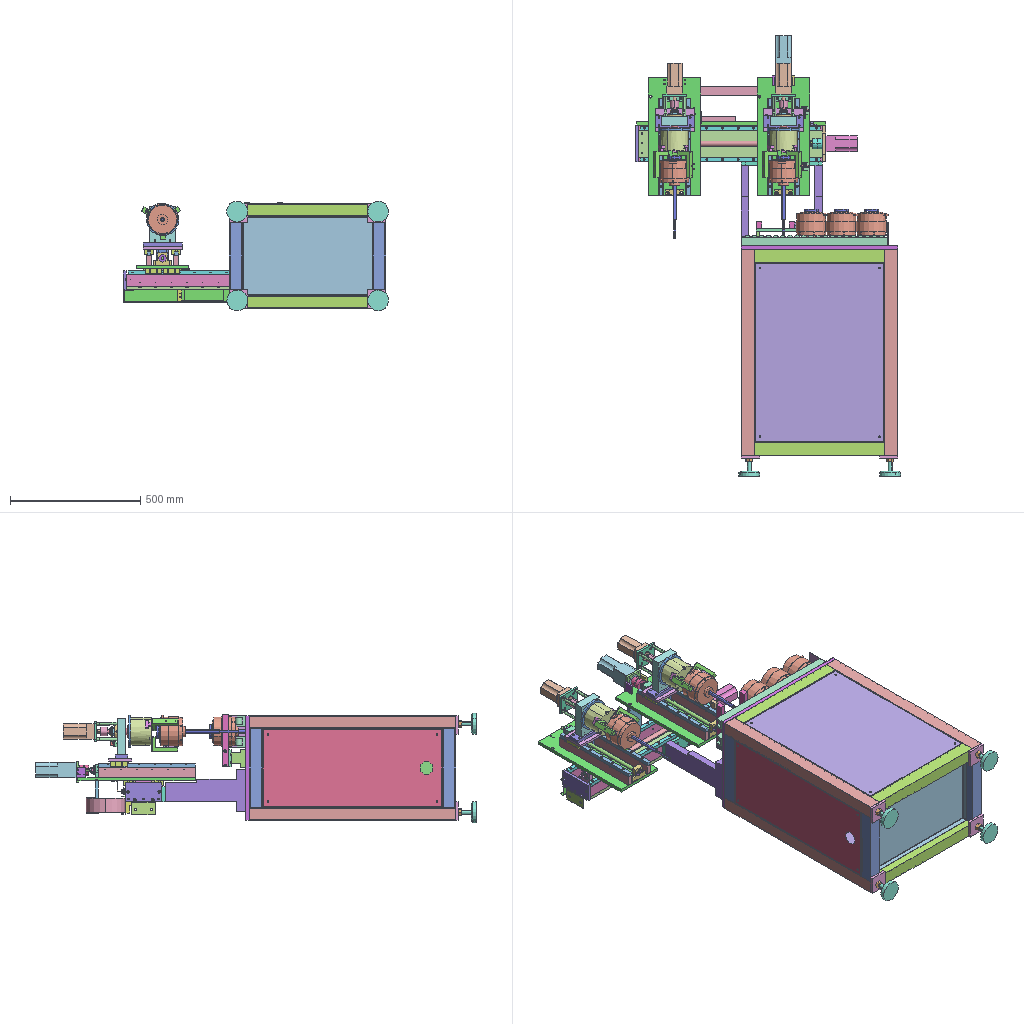Assembly | STEP file | 92 different items | 221 placed | box 1016 x 1690 x 420 mm
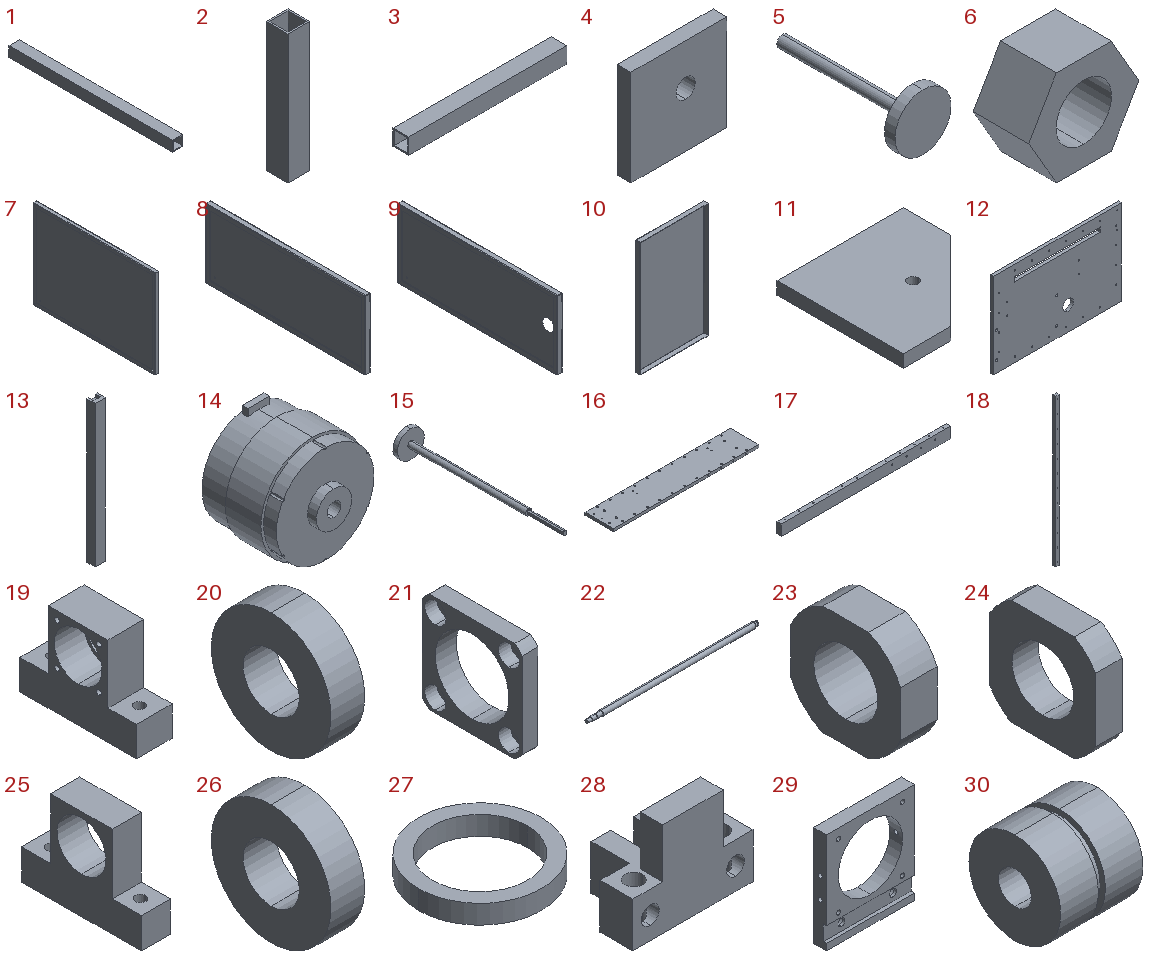Parts list (item | name | quantity | parent item | size | volume):
1 | PN_0082 pillar | x4 | in PN_0002 conveyor frame | 50 x 790 x 50 mm | 581440 mm3
2 | PN_0083 straight stop bar | x4 | in PN_0002 conveyor frame | 50 x 50 x 300 mm | 220800 mm3
3 | PN_0084 cross stop bar | x4 | in PN_0002 conveyor frame | 500 x 50 x 50 mm | 368000 mm3
4 | PN_0078 foot-support plate | x4 | in PN_0024 foot-support plate assembly, conveyor frame | 70 x 10 x 70 mm | 47461 mm3
5 | PN_0079 M16x200 foot pad | x4 | in PN_0024 foot-support plate assembly, conveyor frame | 80 x 200 x 80 mm | 130963 mm3
6 | PN_0077 M16 nut | x4 | in PN_0024 foot-support plate assembly, conveyor frame | 27.713 x 14 x 24 mm | 4828 mm3
7 | PN_0076 front door | x2 | in PN_0002 conveyor frame | 20 x 687 x 497 mm | 627548 mm3
8 | PN_0074 front door | x1 | in PN_0002 conveyor frame | 21.5 x 687 x 297 mm | 405902 mm3
9 | PN_0075 front door | x1 | in PN_0002 conveyor frame | 21.5 x 687 x 297 mm | 402956 mm3
10 | PN_0072 base plate | x1 | in PN_0002 conveyor frame | 300 x 20 x 500 mm | 267366 mm3
11 | PN_0073 sheet-metal fixing block | x16 | in PN_0002 conveyor frame | 40 x 40 x 4 mm | 5116 mm3
12 | PN_0071 table plate | x1 | - | 600 x 14 x 400 mm | 3201054 mm3
13 | PN_0069 wheel-type conveyor belt | x2 | - | 40 x 39.5 x 560 mm | 671037 mm3
14 | PN_0070 stator | x5 | in PN_0067 product | 116 x 98 x 120 mm | 586421 mm3
15 | PN_0068 stator shaft | x5 | in PN_0067 product | 53 x 313.9 x 53 mm | 49554 mm3
16 | PN_0085 crossbeam | x1 | in PN_0002 traverse assembly | 705 x 138 x 13 mm | 1239081 mm3
17 | PN_0086 guide rail spacer block | x2 | in PN_0002 traverse assembly | 705 x 18 x 45 mm | 564305 mm3
18 | PN_0081 15 guide rail, X crossbeam | x2 | in PN_0002 traverse assembly | 15 x 14 x 690 mm | 140414 mm3
19 | PN_0080 main end seat | x1 | in PN_0002 traverse lead screw assembly | 24 x 78 x 59.5 mm | 55003 mm3
20 | PN_0091 bearing ZZB7002 | x2 | in PN_0002 traverse lead screw assembly | 9 x 32 x 32 mm | 5648 mm3
21 | PN_0056 pressing block | x1 | in PN_0002 traverse lead screw assembly | 8 x 38 x 38 mm | 4246 mm3
22 | PN_0055 lead screw 20-5T3 | x1 | in PN_0002 traverse lead screw assembly | 638 x 20 x 20 mm | 189984 mm3
23 | PN_0054 locking nut | x1 | in PN_0002 traverse lead screw assembly | 10 x 24 x 24 mm | 3121 mm3
24 | PN_0053 locking nut | x1 | in PN_0002 traverse lead screw assembly | 6 x 24 x 24 mm | 2302 mm3
25 | PN_0052 secondary end seat | x1 | in PN_0002 traverse lead screw assembly | 19 x 78 x 59.5 mm | 42927 mm3
26 | PN_0090 bearing ZZ6002 | x1 | in PN_0002 traverse lead screw assembly | 9 x 32 x 32 mm | 5648 mm3
27 | PN_0051 retaining ring | x1 | in PN_0002 traverse lead screw assembly | 19.5 x 19.5 x 3 mm | 365.799 mm3
28 | PN_0024 EE-SX-671 photoelectric switch | x4 | in PN_0002 traverse assembly | 26.8 x 15.8 x 21 mm | 3068 mm3
29 | PN_0050 motor plate | x1 | in PN_0024 Z-axis motor assembly | 68 x 10 x 78 mm | 29708 mm3
30 | PN_0049 single diaphragm coupling 39-35-10-14 | x1 | in PN_0024 Z-axis motor assembly | 35 x 39 x 39 mm | 37081 mm3
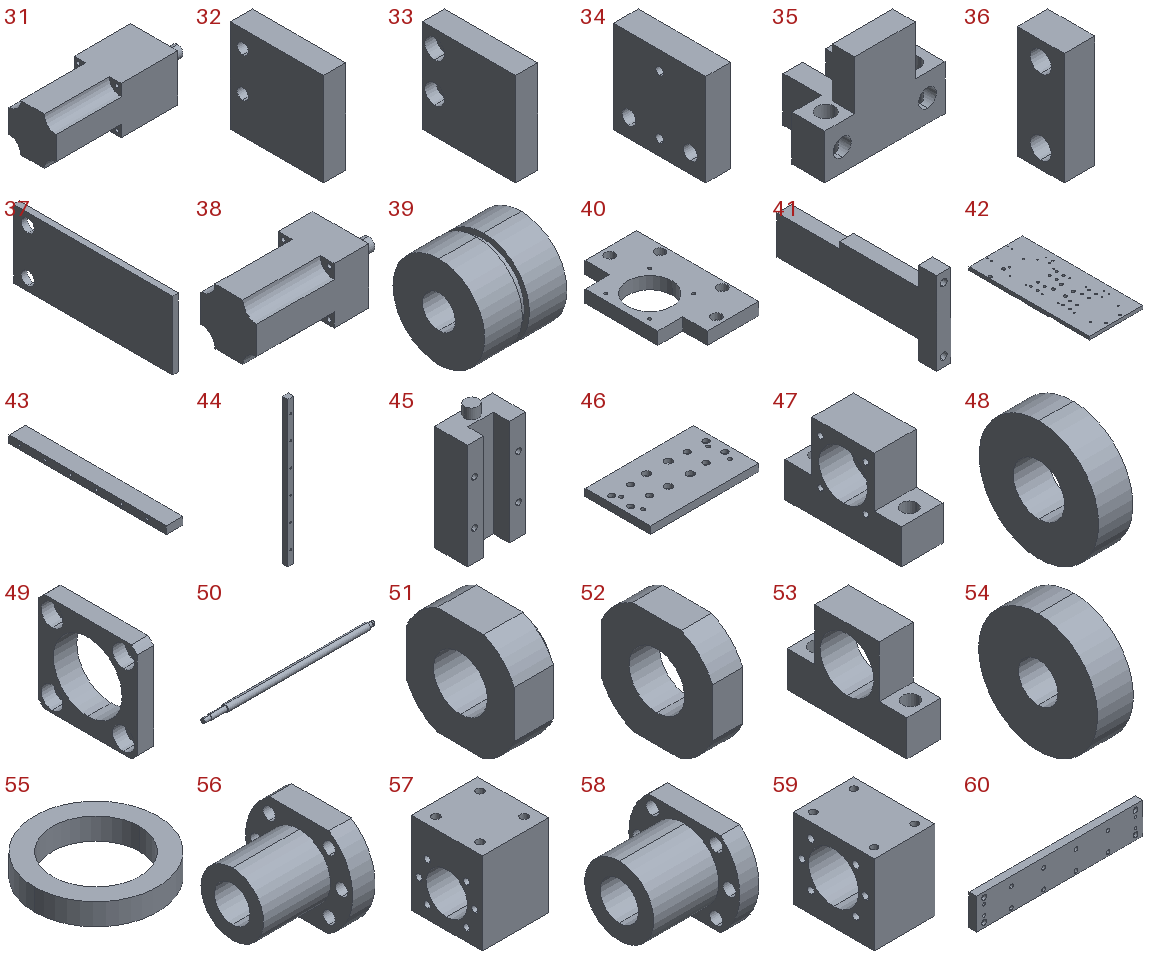31 | PN_0048 MSMD042G, with brake | x1 | in PN_0024 Z-axis motor assembly | 185 x 60 x 60 mm | 504591 mm3
32 | PN_0047 motor plate support | x1 | in PN_0024 Z-axis motor assembly | 9 x 38 x 38 mm | 12038 mm3
33 | PN_0046 motor plate support | x1 | in PN_0024 Z-axis motor assembly | 9 x 38 x 38 mm | 12038 mm3
34 | PN_0045 fixing block | x2 | in PN_0024 sensor assembly | 8 x 30 x 30 mm | 6551 mm3
35 | PN_0010 EE-SX-671 photoelectric switch | x2 | in PN_0024 sensor assembly | 26.8 x 15.8 x 21 mm | 3068 mm3
36 | PN_0044 spacer | x1 | in PN_0024 spacer assembly | 6.5 x 10 x 24 mm | 1353 mm3
37 | PN_0043 sensor plate | x1 | in PN_0024 spacer assembly | 2 x 56 x 24 mm | 2624 mm3
38 | PN_0048 MSMD042G | x1 | in PN_0024 traverse motor assembly | 150 x 60 x 60 mm | 380918 mm3
39 | PN_0042 single diaphragm coupling 39-35-14-12 | x1 | in PN_0024 traverse motor assembly | 35 x 39 x 39 mm | 36443 mm3
40 | PN_0041 motor spacer block | x1 | in PN_0024 traverse motor assembly | 86 x 138 x 14 mm | 112662 mm3
41 | PN_0014 spacer block | x2 | in PN_0002 crossbeam assembly | 28 x 308 x 160 mm | 760293 mm3
42 | PN_0040 Z-axis plate | x2 | in PN_0002 Z-axis assembly | 200 x 450 x 12 mm | 1035466 mm3
43 | PN_0039 spacer plate | x4 | in PN_0002 Z-axis assembly | 39 x 370 x 18 mm | 248718 mm3
44 | PN_0038 15 guide rail | x4 | in PN_0002 Z-axis assembly | 15 x 14 x 370 mm | 75457 mm3
45 | PN_0037 15 square slider, H=24 | x12 | in PN_0002 Z-axis assembly | 34 x 19.4 x 68 mm | 31791 mm3
46 | PN_0036 moving plate | x2 | in PN_0002 Z-axis assembly | 150 x 90 x 10 mm | 129300 mm3
47 | PN_0035 main end seat | x2 | in PN_0002 Z-axis lead screw assembly | 24 x 67 x 49 mm | 40517 mm3
48 | PN_0089 bearing ZZB7001 | x4 | in PN_0002 Z-axis lead screw assembly | 8 x 28 x 28 mm | 4021 mm3
49 | PN_0034 pressing block | x2 | in PN_0002 Z-axis lead screw assembly | 8.5 x 36 x 36 mm | 4077 mm3
50 | PN_0033 lead screw 16-5T3 | x2 | in PN_0002 Z-axis lead screw assembly | 418 x 16 x 16 mm | 77018 mm3
51 | PN_0032 locking nut | x2 | in PN_0002 Z-axis lead screw assembly | 11 x 22 x 22 mm | 2971 mm3
52 | PN_0031 locking nut | x2 | in PN_0002 Z-axis lead screw assembly | 6 x 22 x 22 mm | 1989 mm3
53 | PN_0030 secondary end seat | x2 | in PN_0002 Z-axis lead screw assembly | 19 x 67 x 49 mm | 29321 mm3
54 | PN_0088 bearing ZZ6200 | x2 | in PN_0002 Z-axis lead screw assembly | 9 x 30 x 30 mm | 5655 mm3
55 | PN_0029 retaining ring | x2 | in PN_0002 Z-axis lead screw assembly | 17 x 17 x 3 mm | 341.648 mm3
56 | PN_0028 16-5T3 nut | x2 | in PN_0024 Z-axis nut assembly | 40 x 48 x 40 mm | 25660 mm3
57 | PN_0027 nut block | x2 | in PN_0024 Z-axis nut assembly | 45 x 48 x 56 mm | 90968 mm3
58 | PN_0026 20-5T3 nut | x2 | in PN_0024 traverse nut | 44 x 58 x 44 mm | 41531 mm3
59 | PN_0025 nut block | x2 | in PN_0024 traverse nut | 45 x 60 x 59 mm | 107872 mm3
60 | PN_0023 base plate | x1 | in PN_0002 crossbeam assembly | 310 x 14 x 58 mm | 238676 mm3
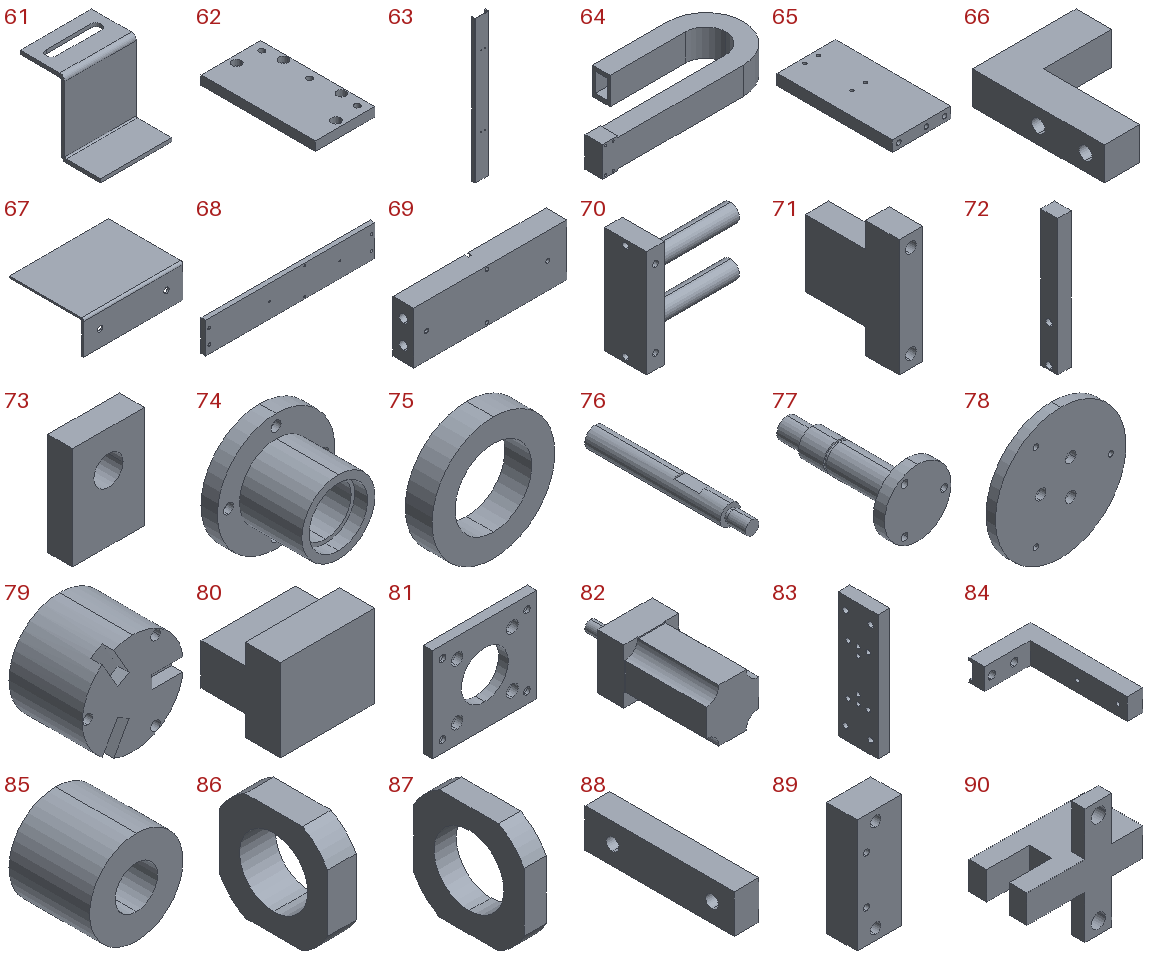61 | PN_0022 sensor plate | x2 | in PN_0002 crossbeam assembly | 40 x 45 x 42 mm | 6324 mm3
62 | PN_0021 cover block | x1 | in PN_0002 crossbeam assembly | 72 x 138 x 11 mm | 104938 mm3
63 | PN_0020 tank-chain support plate | x1 | in PN_0002 crossbeam assembly | 69 x 18 x 725 mm | 144131 mm3
64 | PN_0019 tank chain, outer 35x54, inner 25x38 | x1 | in PN_0002 crossbeam assembly | 355 x 150 x 60 mm | 607044 mm3
65 | PN_0018 tank-chain fixing block | x1 | in PN_0002 crossbeam assembly | 64 x 126 x 12 mm | 95444 mm3
66 | PN_0017 fixing block | x2 | in PN_0002 crossbeam assembly | 44 x 56 x 14 mm | 16926 mm3
67 | PN_0016 stop plate | x1 | - | 120 x 90 x 40 mm | 30408 mm3
68 | PN_0015 spacer block | x1 | in PN_0002 material-push cylinder assembly | 350 x 10 x 64 mm | 221459 mm3
69 | PN_0014 cylinder TN-20X125 | x1 | in PN_0002 TN20-20 cylinder assembly | 183 x 25 x 62 mm | 276727 mm3
70 | PN_0013 cylinder TN-20X125 | x1 | in PN_0002 TN20-20 cylinder assembly | 60 x 24 x 61 mm | 21912 mm3
71 | PN_0057 cylinder spacer block | x2 | in PN_0002 material-push cylinder assembly | 14 x 56 x 70 mm | 38077 mm3
72 | PN_0058 push block | x2 | in PN_0002 material-push cylinder assembly | 20 x 25 x 200 mm | 98425 mm3
73 | PN_0012 connecting plate | x2 | in PN_0002 claw assembly | 98 x 34 x 140 mm | 419089 mm3
74 | PN_0011 shaft seat | x2 | in PN_0002 claw assembly | 64 x 43 x 64 mm | 40458 mm3
75 | PN_0087 bearing ZZ6804 | x4 | in PN_0002 claw assembly | 32 x 7 x 32 mm | 3431 mm3
76 | PN_0059 pillar | x8 | in PN_0002 claw assembly | 12 x 93 x 12 mm | 9356 mm3
77 | PN_0060 rotating shaft | x2 | in PN_0002 claw assembly | 48 x 94 x 48 mm | 39121 mm3
78 | PN_0061 fixing block | x2 | in PN_0002 claw assembly | 124 x 9 x 124 mm | 101363 mm3
79 | PN_0062 gripper MHS3-80D | x2 | in PN_0010 MH3-80D gripper | 106 x 77 x 106 mm | 654143 mm3
80 | PN_0009 gripper MHS3-80D | x6 | in PN_0010 MH3-80D gripper | 32 x 27 x 28 mm | 16863 mm3
81 | PN_0008 motor plate | x2 | in PN_0010 rotary motor assembly | 89 x 8 x 80 mm | 42888 mm3
82 | PN_0007 planetary reduction stepper motor PLX60-L1-7 | x2 | in PN_0010 rotary motor assembly | 60 x 155.5 x 60 mm | 360183 mm3
83 | PN_0064 fixing plate | x2 | in PN_0002 claw assembly | 14 x 48 x 150 mm | 95205 mm3
84 | PN_0063 gripper jaw | x6 | in PN_0002 claw assembly | 54 x 100 x 19 mm | 33980 mm3
85 | PN_0065 single diaphragm coupling | x2 | in PN_0002 claw assembly | 33 x 28.5 x 33 mm | 20198 mm3
86 | PN_0006 nut | x2 | in PN_0002 claw assembly | 10 x 30 x 30 mm | 4642 mm3
87 | PN_0005 nut | x2 | in PN_0002 claw assembly | 6 x 30 x 30 mm | 3228 mm3
88 | PN_0004 rubber pad | x6 | in PN_0002 claw assembly | 9 x 54 x 14 mm | 6202 mm3
89 | PN_0003 sensor seat | x2 | in PN_0010 rotary zero-position assembly | 19 x 13 x 49 mm | 11246 mm3
90 | PN_0010 photoelectric switch EE-SX672, Omron | x2 | in PN_0010 rotary zero-position assembly | 26 x 13 x 26 mm | 2136 mm3
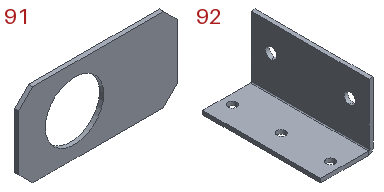91 | PN_0066 sensor plate | x2 | in PN_0002 claw assembly | 57 x 1.5 x 30 mm | 1970 mm3
92 | PN_0001 connector code | x1 | - | 40 x 90 x 50 mm | 22592 mm3
Placements (level | parent | child | x y z in mm | rotation matrix by rows):
1 | subassembly 2 | PN_0002 conveyor frame | 537.353 771.982 125.0 | 1 0 0 0 1 0 0 0 1
2 | PN_0002 conveyor frame | PN_0082 pillar | -72.682 -1094.173 -0.0 | 1 0 0 0 1 0 0 0 1
2 | PN_0002 conveyor frame | PN_0083 straight stop bar | -72.682 -329.173 -325.0 | 1 0 0 0 1 0 0 0 1
2 | PN_0002 conveyor frame | PN_0082 pillar | -72.682 -1094.173 -350.0 | 1 0 0 0 1 0 0 0 1
2 | PN_0002 conveyor frame | PN_0084 cross stop bar | -597.682 -329.173 -0.0 | 1 0 0 0 1 0 0 0 1
2 | PN_0002 conveyor frame | PN_0082 pillar | -622.682 -1094.173 -0.0 | 1 0 0 0 1 0 0 0 1
2 | PN_0002 conveyor frame | PN_0082 pillar | -622.682 -1094.173 -350.0 | 1 0 0 0 1 0 0 0 1
2 | PN_0002 conveyor frame | PN_0084 cross stop bar | -597.682 -329.173 -350.0 | 1 0 0 0 1 0 0 0 1
2 | PN_0002 conveyor frame | PN_0083 straight stop bar | -622.682 -329.173 -325.0 | 1 0 0 0 1 0 0 0 1
2 | PN_0002 conveyor frame | PN_0084 cross stop bar | -597.682 -1069.173 -0.0 | 1 0 0 0 1 0 0 0 1
2 | PN_0002 conveyor frame | PN_0084 cross stop bar | -597.682 -1069.173 -350.0 | 1 0 0 0 1 0 0 0 1
2 | PN_0002 conveyor frame | PN_0024 foot-support plate assembly, conveyor frame | -1.742 -1099.218 -50.0 | 1 0 0 0 1 0 0 0 1
3 | PN_0024 foot-support plate assembly, conveyor frame | PN_0078 foot-support plate | -45.94 -4.955 75.0 | 1 0 0 0 1 0 0 0 1
3 | PN_0024 foot-support plate assembly, conveyor frame | PN_0079 M16x200 foot pad | -75.94 -74.955 45.0 | 0.8587 0 0.5125 0 1 0 -0.5125 0 0.8587
3 | PN_0024 foot-support plate assembly, conveyor frame | PN_0077 M16 nut | -75.94 -18.955 45.0 | 1 0 0 0 1 0 0 0 1
2 | PN_0002 conveyor frame | PN_0024 foot-support plate assembly, conveyor frame | -572.682 -1099.218 70.94 | 0 0 -1 0 1 0 1 0 0
3 | PN_0024 foot-support plate assembly, conveyor frame | PN_0078 foot-support plate | -45.94 -4.955 75.0 | 1 0 0 0 1 0 0 0 1
3 | PN_0024 foot-support plate assembly, conveyor frame | PN_0079 M16x200 foot pad | -75.94 -74.955 45.0 | 0.8587 0 0.5125 0 1 0 -0.5125 0 0.8587
3 | PN_0024 foot-support plate assembly, conveyor frame | PN_0077 M16 nut | -75.94 -18.955 45.0 | 1 0 0 0 1 0 0 0 1
2 | PN_0002 conveyor frame | PN_0024 foot-support plate assembly, conveyor frame | -693.622 -1099.218 -300.0 | -1 0 0 0 1 0 0 0 -1
3 | PN_0024 foot-support plate assembly, conveyor frame | PN_0078 foot-support plate | -45.94 -4.955 75.0 | 1 0 0 0 1 0 0 0 1
3 | PN_0024 foot-support plate assembly, conveyor frame | PN_0079 M16x200 foot pad | -75.94 -74.955 45.0 | 0.8587 0 0.5125 0 1 0 -0.5125 0 0.8587
3 | PN_0024 foot-support plate assembly, conveyor frame | PN_0077 M16 nut | -75.94 -18.955 45.0 | 1 0 0 0 1 0 0 0 1
2 | PN_0002 conveyor frame | PN_0024 foot-support plate assembly, conveyor frame | -122.682 -1099.218 -420.94 | 0 0 1 0 1 0 -1 0 0
3 | PN_0024 foot-support plate assembly, conveyor frame | PN_0078 foot-support plate | -45.94 -4.955 75.0 | 1 0 0 0 1 0 0 0 1
3 | PN_0024 foot-support plate assembly, conveyor frame | PN_0079 M16x200 foot pad | -75.94 -74.955 45.0 | 0.8587 0 0.5125 0 1 0 -0.5125 0 0.8587
3 | PN_0024 foot-support plate assembly, conveyor frame | PN_0077 M16 nut | -75.94 -18.955 45.0 | 1 0 0 0 1 0 0 0 1
2 | PN_0002 conveyor frame | PN_0083 straight stop bar | -72.682 -1069.173 -325.0 | 1 0 0 0 1 0 0 0 1
2 | PN_0002 conveyor frame | PN_0083 straight stop bar | -622.682 -1069.173 -325.0 | 0 -1 0 1 0 0 0 0 1
2 | PN_0002 conveyor frame | PN_0076 front door | -347.682 -699.173 25.0 | 0 0 -1 0 1 0 1 0 0
2 | PN_0002 conveyor frame | PN_0074 front door | -47.682 -699.173 -175.0 | 1 0 0 0 1 0 0 0 1
2 | PN_0002 conveyor frame | PN_0075 front door | -647.682 -699.173 -175.0 | -1 0 0 0 1 0 0 0 -1
2 | PN_0002 conveyor frame | PN_0076 front door | -347.682 -699.173 -375.0 | 0 0 1 0 1 0 -1 0 -0
2 | PN_0002 conveyor frame | PN_0072 base plate | -347.682 -1044.173 -175.0 | 0 0 1 0 1 0 -1 0 0
2 | PN_0002 conveyor frame | PN_0073 sheet-metal fixing block | -597.682 -354.173 -351.0 | 1 0 0 0 1 0 0 0 1
2 | PN_0002 conveyor frame | PN_0073 sheet-metal fixing block | -97.682 -354.173 -351.0 | 0 1 0 -1 0 0 0 0 1
2 | PN_0002 conveyor frame | PN_0073 sheet-metal fixing block | -97.682 -1044.173 -351.0 | -1 0 0 0 -1 0 0 0 1
2 | PN_0002 conveyor frame | PN_0073 sheet-metal fixing block | -597.682 -1044.173 -351.0 | 0 -1 0 1 0 0 0 0 1
2 | PN_0002 conveyor frame | PN_0073 sheet-metal fixing block | -97.682 -354.173 1.0 | 0 1 0 -1 0 0 0 0 1
2 | PN_0002 conveyor frame | PN_0073 sheet-metal fixing block | -597.682 -354.173 1.0 | 1 0 0 0 1 0 0 0 1
2 | PN_0002 conveyor frame | PN_0073 sheet-metal fixing block | -597.682 -1044.173 1.0 | 0 -1 0 1 0 0 0 0 1
2 | PN_0002 conveyor frame | PN_0073 sheet-metal fixing block | -97.682 -1044.173 1.0 | -1 0 0 0 -1 0 0 0 1
2 | PN_0002 conveyor frame | PN_0073 sheet-metal fixing block | -623.682 -1044.173 -325.0 | 0 0 -1 1 0 0 0 -1 0
2 | PN_0002 conveyor frame | PN_0073 sheet-metal fixing block | -623.682 -1044.173 -25.0 | 0 0 1 1 0 0 0 1 -0
2 | PN_0002 conveyor frame | PN_0073 sheet-metal fixing block | -623.682 -354.173 -25.0 | 0 0 1 0 1 0 -1 0 -0
2 | PN_0002 conveyor frame | PN_0073 sheet-metal fixing block | -623.682 -354.173 -325.0 | 0 0 1 -1 0 0 0 -1 -0
2 | PN_0002 conveyor frame | PN_0073 sheet-metal fixing block | -71.682 -1044.173 -325.0 | 0 0 -1 1 0 0 0 -1 0
2 | PN_0002 conveyor frame | PN_0073 sheet-metal fixing block | -71.682 -1044.173 -25.0 | 0 0 -1 0 -1 0 -1 0 0
2 | PN_0002 conveyor frame | PN_0073 sheet-metal fixing block | -71.682 -354.173 -325.0 | 0 0 1 -1 0 0 0 -1 -0
2 | PN_0002 conveyor frame | PN_0073 sheet-metal fixing block | -71.682 -354.173 -25.0 | 0 0 1 0 1 0 -1 0 0
1 | subassembly 2 | PN_0071 table plate | 189.671 467.809 -50.0 | 1 0 0 0 1 0 0 0 1
1 | subassembly 2 | PN_0069 wheel-type conveyor belt | -110.329 481.809 130.0 | 0 0 -1 0 1 0 1 0 -0
1 | subassembly 2 | PN_0069 wheel-type conveyor belt | -110.329 481.809 50.0 | 0 0 -1 0 1 0 1 0 -0
1 | subassembly 2 | PN_0067 product | 166.59 553.419 70.693 | 0.3432 0 0.9393 0 1 0 -0.9393 0 0.3432
2 | PN_0067 product | PN_0070 stator | -21.286 -42.11 -2.0 | 1 0 0 0 1 0 0 0 1
2 | PN_0067 product | PN_0068 stator shaft | -21.286 -245.41 -2.0 | -0.9481 0 0.3179 0 1 0 -0.3179 0 -0.9481
1 | subassembly 2 | PN_0002 crossbeam assembly | 735.783 672.136 -112.134 | 1 0 0 0 0.9998 -0.01827 0 0.01827 0.9998
2 | PN_0002 crossbeam assembly | PN_0002 traverse assembly | -832.649 207.181 -64.162 | 1 0 0 0 0.9998 0.01827 0 -0.01827 0.9998
3 | PN_0002 traverse assembly | PN_0085 crossbeam | -55.963 -7.645 0.0 | 1 0 0 0 1 0 0 0 1
3 | PN_0002 traverse assembly | PN_0086 guide rail spacer block | -55.963 52.355 6.5 | 1 0 0 0 1 0 0 0 1
3 | PN_0002 traverse assembly | PN_0086 guide rail spacer block | -55.963 -67.645 6.5 | 1 0 0 0 1 0 0 0 1
3 | PN_0002 traverse assembly | PN_0081 15 guide rail, X crossbeam | -400.963 52.355 51.5 | 0 0 -1 -1 0 0 0 1 -0
3 | PN_0002 traverse assembly | PN_0081 15 guide rail, X crossbeam | -400.963 -67.645 51.5 | 0 0 -1 -1 0 0 0 1 0
3 | PN_0002 traverse assembly | PN_0002 traverse lead screw assembly | 111.942 -25.688 33.5 | -1 0 0 0 -1 0 0 0 1
4 | PN_0002 traverse lead screw assembly | PN_0080 main end seat | -115.595 -18.043 -27.0 | 1 0 0 0 1 0 0 0 1
4 | PN_0002 traverse lead screw assembly | PN_0091 bearing ZZB7002 | -112.095 -18.043 13.0 | 1 0 0 0 1 0 0 0 1
4 | PN_0002 traverse lead screw assembly | PN_0091 bearing ZZB7002 | -121.095 -18.043 13.0 | 1 0 0 0 0.9947 0.1024 0 -0.1024 0.9947
4 | PN_0002 traverse lead screw assembly | PN_0056 pressing block | -125.595 -18.043 13.0 | 1 0 0 0 1 0 0 0 1
4 | PN_0002 traverse lead screw assembly | PN_0055 lead screw 20-5T3 | 476.405 -18.043 13.0 | 1 0 0 0 0.03395 -0.9994 0 0.9994 0.03395
4 | PN_0002 traverse lead screw assembly | PN_0054 locking nut | -128.595 -18.043 13.0 | 1 0 0 0 0.02104 0.9998 0 -0.9998 0.02104
4 | PN_0002 traverse lead screw assembly | PN_0053 locking nut | -138.595 -18.043 13.0 | 1 0 0 0 1 0 0 0 1
4 | PN_0002 traverse lead screw assembly | PN_0052 secondary end seat | 466.905 -18.043 -27.0 | 1 0 0 0 1 0 0 0 1
4 | PN_0002 traverse lead screw assembly | PN_0090 bearing ZZ6002 | 466.905 -18.043 13.0 | 1 0 0 0 1 0 0 0 1
4 | PN_0002 traverse lead screw assembly | PN_0051 retaining ring | -128.595 -18.043 13.0 | 0 0 1 0 1 0 -1 0 -0
3 | PN_0002 traverse assembly | PN_0024 EE-SX-671 photoelectric switch | 236.537 61.355 32.5 | 0 0 -1 0 1 0 1 0 -0
3 | PN_0002 traverse assembly | PN_0024 EE-SX-671 photoelectric switch | -288.463 61.355 32.5 | 0 0 1 0 1 0 -1 0 -0
3 | PN_0002 traverse assembly | PN_0024 EE-SX-671 photoelectric switch | -308.463 61.355 32.5 | 0 0 -1 0 1 0 1 0 -0
3 | PN_0002 traverse assembly | PN_0024 EE-SX-671 photoelectric switch | 256.537 61.355 32.5 | 0 0 1 0 1 0 -1 0 -0
2 | PN_0002 crossbeam assembly | PN_0024 Z-axis motor assembly | -612.442 468.818 39.577 | 1 0 0 0 0.9998 0.01827 0 -0.01827 0.9998
3 | PN_0024 Z-axis motor assembly | PN_0050 motor plate | -72.171 -17.844 -40.0 | 1 0 0 0 1 0 0 0 1
3 | PN_0024 Z-axis motor assembly | PN_0049 single diaphragm coupling 39-35-10-14 | -72.171 -39.344 6.0 | 0 -0.9981 -0.06184 -1 0 0 0 0.06184 -0.9981
3 | PN_0024 Z-axis motor assembly | PN_0048 MSMD042G, with brake | -72.171 -7.844 6.0 | 0 1 0 -1 0 0 0 0 1
3 | PN_0024 Z-axis motor assembly | PN_0047 motor plate support | -33.67 -7.844 -23.0 | 1 0 0 0 1 0 0 0 1
3 | PN_0024 Z-axis motor assembly | PN_0046 motor plate support | -110.671 -7.844 -23.0 | 1 0 0 0 1 0 0 0 1
2 | PN_0002 crossbeam assembly | PN_0024 sensor assembly | -601.612 328.757 89.809 | 0 0 1 0.01827 -0.9998 0 0.9998 0.01827 0
3 | PN_0024 sensor assembly | PN_0045 fixing block | -70.666 -0.6116 -15.0 | 1 0 0 0 1 0 0 0 1
3 | PN_0024 sensor assembly | PN_0010 EE-SX-671 photoelectric switch | -62.666 -0.6116 -0.5 | 0 1 0 0 0 -1 -1 0 -0
2 | PN_0002 crossbeam assembly | PN_0024 sensor assembly | -601.612 113.793 93.737 | 0 0 1 0.01827 -0.9998 0 0.9998 0.01827 0
3 | PN_0024 sensor assembly | PN_0045 fixing block | -70.666 -0.6116 -15.0 | 1 0 0 0 1 0 0 0 1
3 | PN_0024 sensor assembly | PN_0010 EE-SX-671 photoelectric switch | -62.666 -0.6116 -0.5 | 0 1 0 0 0 -1 -1 0 -0
2 | PN_0002 crossbeam assembly | PN_0024 spacer assembly | -529.966 310.611 96.038 | 1 0 0 0 0.01827 -0.9998 0 0.9998 0.01827
3 | PN_0024 spacer assembly | PN_0044 spacer | -79.646 -13.563 -0.0 | 1 0 0 0 1 0 0 0 1
3 | PN_0024 spacer assembly | PN_0043 sensor plate | -73.146 -59.563 -0.0 | 1 0 0 0 1 0 0 0 1
2 | PN_0002 crossbeam assembly | PN_0024 traverse motor assembly | -2000.11 -7.077 11.568 | -1 0 0 0 0.9934 -0.1144 0 -0.1144 -0.9934
3 | PN_0024 traverse motor assembly | PN_0048 MSMD042G | -1477.998 209.43 5.172 | 1 0 0 0 -0.09624 0.9954 0 -0.9954 -0.09624
3 | PN_0024 traverse motor assembly | PN_0042 single diaphragm coupling 39-35-14-12 | -1445.498 209.43 5.172 | 1 0 0 0 1 -0.001195 0 0.001195 1
3 | PN_0024 traverse motor assembly | PN_0041 motor spacer block | -1463.998 206.35 -26.679 | 0 0 -1 0.09624 0.9954 0 0.9954 -0.09624 -0
2 | PN_0002 crossbeam assembly | PN_0014 spacer block | -550.112 -190.731 -20.386 | 1 0 0 0 0.9998 0.01827 0 -0.01827 0.9998
2 | PN_0002 crossbeam assembly | PN_0014 spacer block | -832.112 -190.731 -20.386 | 1 0 0 0 0.9998 0.01827 0 -0.01827 0.9998
2 | PN_0002 crossbeam assembly | PN_0002 Z-axis assembly | -705.13 171.828 15.998 | 1 0 0 0 0.9998 0.01827 0 -0.01827 0.9998
3 | PN_0002 Z-axis assembly | PN_0040 Z-axis plate | 20.518 -168.834 -0.0 | 1 0 0 0 1 0 0 0 1
3 | PN_0002 Z-axis assembly | PN_0039 spacer plate | 72.518 -168.834 6.0 | 0 0 -1 0 1 0 1 0 -0
3 | PN_0002 Z-axis assembly | PN_0039 spacer plate | -31.482 -168.834 6.0 | 0 0 -1 0 1 0 1 0 -0
3 | PN_0002 Z-axis assembly | PN_0038 15 guide rail | -31.482 -168.834 45.0 | 1 0 0 0 0 -1 0 1 -0
3 | PN_0002 Z-axis assembly | PN_0038 15 guide rail | 72.518 -168.834 45.0 | 1 0 0 0 0 -1 0 1 -0
3 | PN_0002 Z-axis assembly | PN_0037 15 square slider, H=24 | -31.482 124.166 49.6 | 1 0 0 0 0 -1 0 1 -0
3 | PN_0002 Z-axis assembly | PN_0037 15 square slider, H=24 | 72.518 124.166 49.6 | 1 0 0 0 0 -1 0 1 -0
3 | PN_0002 Z-axis assembly | PN_0036 moving plate | 20.518 74.166 74.0 | 1 0 0 0 1 0 0 0 1
3 | PN_0002 Z-axis assembly | PN_0002 Z-axis lead screw assembly | 38.561 88.071 33.0 | 0 1 0 -1 0 0 0 0 1
4 | PN_0002 Z-axis lead screw assembly | PN_0035 main end seat | -115.595 -18.043 -27.0 | 1 0 0 0 1 0 0 0 1
4 | PN_0002 Z-axis lead screw assembly | PN_0089 bearing ZZB7001 | -113.595 -18.043 2.0 | 1 0 0 0 1 0 0 0 1
4 | PN_0002 Z-axis lead screw assembly | PN_0089 bearing ZZB7001 | -121.595 -18.043 2.0 | 1 0 0 0 0.9947 0.1024 0 -0.1024 0.9947
4 | PN_0002 Z-axis lead screw assembly | PN_0034 pressing block | -125.595 -18.043 2.0 | 1 0 0 0 1 0 0 0 1
4 | PN_0002 Z-axis lead screw assembly | PN_0033 lead screw 16-5T3 | 254.405 -18.043 2.0 | 1 0 0 0 -0.119 0.9929 0 -0.9929 -0.119
4 | PN_0002 Z-axis lead screw assembly | PN_0032 locking nut | -128.595 -18.043 2.0 | 1 0 0 0 -0.07717 0.997 0 -0.997 -0.07717
4 | PN_0002 Z-axis lead screw assembly | PN_0031 locking nut | -139.595 -18.043 2.0 | 1 0 0 0 1 0.004162 0 -0.004162 1
4 | PN_0002 Z-axis lead screw assembly | PN_0030 secondary end seat | 244.905 -18.043 -27.0 | 1 0 0 0 1 0 0 0 1
4 | PN_0002 Z-axis lead screw assembly | PN_0088 bearing ZZ6200 | 244.905 -18.043 2.0 | 1 0 0 0 1 0 0 0 1
4 | PN_0002 Z-axis lead screw assembly | PN_0029 retaining ring | -125.595 -18.043 2.0 | 0 0 -1 0.5089 0.8608 0 0.8608 -0.5089 -0
3 | PN_0002 Z-axis assembly | PN_0024 Z-axis nut assembly | 38.561 71.285 33.0 | 0 1 0 -1 0 0 0 0 1
4 | PN_0024 Z-axis nut assembly | PN_0028 16-5T3 nut | -85.381 -18.043 2.0 | -1 0 0 0 1 0 0 0 -1
4 | PN_0024 Z-axis nut assembly | PN_0027 nut block | -52.881 -18.043 -20.0 | 1 0 0 0 1 0 0 0 1
3 | PN_0002 Z-axis assembly | PN_0037 15 square slider, H=24 | 55.518 89.166 -23.4 | 0 0 1 1 0 0 0 1 -0
3 | PN_0002 Z-axis assembly | PN_0037 15 square slider, H=24 | 55.518 -30.834 -23.4 | 0 0 1 1 0 0 0 1 -0
3 | PN_0002 Z-axis assembly | PN_0037 15 square slider, H=24 | -14.482 89.166 -23.4 | 0 0 -1 -1 0 0 0 1 -0
3 | PN_0002 Z-axis assembly | PN_0037 15 square slider, H=24 | -14.482 -30.834 -23.4 | 0 0 -1 -1 0 0 0 1 0
2 | PN_0002 crossbeam assembly | PN_0024 traverse nut | -643.517 218.189 -30.857 | 1 0 0 0 0.9998 0.01827 0 -0.01827 0.9998
3 | PN_0024 traverse nut | PN_0026 20-5T3 nut | -8.595 -18.043 13.0 | 1 0 0 0 -1 0 0 0 -1
3 | PN_0024 traverse nut | PN_0025 nut block | -41.095 -18.043 -19.0 | -1 0 0 0 -1 0 0 0 1
2 | PN_0002 crossbeam assembly | PN_0023 base plate | -846.112 117.492 -11.014 | 1 0 0 0 0.9998 0.01827 0 -0.01827 0.9998
2 | PN_0002 crossbeam assembly | PN_0022 sensor plate | -619.112 279.136 -31.971 | 1 0 0 0 0.9998 0.01827 0 -0.01827 0.9998
2 | PN_0002 crossbeam assembly | PN_0021 cover block | -1241.112 200.734 1.467 | 0 0 -1 -0.01827 -0.9998 0 -0.9998 0.01827 0
2 | PN_0002 crossbeam assembly | PN_0022 sensor plate | -1019.112 279.136 -31.971 | 1 0 0 0 0.9998 0.01827 0 -0.01827 0.9998
2 | PN_0002 crossbeam assembly | PN_0020 tank-chain support plate | -884.612 270.154 -85.665 | 0 0 1 -0.01827 0.9998 0 -0.9998 -0.01827 0
2 | PN_0002 crossbeam assembly | PN_0019 tank chain, outer 35x54, inner 25x38 | -768.112 420.12 -88.905 | -1 0 0 0 -0.9998 0.01827 0 0.01827 0.9998
2 | PN_0002 crossbeam assembly | PN_0018 tank-chain fixing block | -751.612 380.85 6.178 | 1 0 0 0 -0.01827 0.9998 0 -0.9998 -0.01827
2 | PN_0002 crossbeam assembly | PN_0017 fixing block | -676.112 212.416 -70.758 | 0 0 1 -0.01827 0.9998 0 -0.9998 -0.01827 0
2 | PN_0002 crossbeam assembly | PN_0017 fixing block | -1036.112 212.416 -70.758 | 0 0 1 -0.01827 0.9998 0 -0.9998 -0.01827 0
2 | PN_0002 crossbeam assembly | PN_0024 traverse nut | -1061.017 218.189 -30.857 | 1 0 0 0 0.9998 0.01827 0 -0.01827 0.9998
3 | PN_0024 traverse nut | PN_0026 20-5T3 nut | -8.595 -18.043 13.0 | 1 0 0 0 -1 0 0 0 -1
3 | PN_0024 traverse nut | PN_0025 nut block | -41.095 -18.043 -19.0 | -1 0 0 0 -1 0 0 0 1
2 | PN_0002 crossbeam assembly | PN_0002 Z-axis assembly | -1122.63 171.828 15.998 | 1 0 0 0 0.9998 0.01827 0 -0.01827 0.9998
3 | PN_0002 Z-axis assembly | PN_0040 Z-axis plate | 20.518 -168.834 -0.0 | 1 0 0 0 1 0 0 0 1
3 | PN_0002 Z-axis assembly | PN_0039 spacer plate | 72.518 -168.834 6.0 | 0 0 -1 0 1 0 1 0 -0
3 | PN_0002 Z-axis assembly | PN_0039 spacer plate | -31.482 -168.834 6.0 | 0 0 -1 0 1 0 1 0 -0
3 | PN_0002 Z-axis assembly | PN_0038 15 guide rail | -31.482 -168.834 45.0 | 1 0 0 0 0 -1 0 1 -0
3 | PN_0002 Z-axis assembly | PN_0038 15 guide rail | 72.518 -168.834 45.0 | 1 0 0 0 0 -1 0 1 -0
3 | PN_0002 Z-axis assembly | PN_0037 15 square slider, H=24 | -31.482 124.166 49.6 | 1 0 0 0 0 -1 0 1 -0
3 | PN_0002 Z-axis assembly | PN_0037 15 square slider, H=24 | 72.518 124.166 49.6 | 1 0 0 0 0 -1 0 1 -0
3 | PN_0002 Z-axis assembly | PN_0036 moving plate | 20.518 74.166 74.0 | 1 0 0 0 1 0 0 0 1
3 | PN_0002 Z-axis assembly | PN_0002 Z-axis lead screw assembly | 38.561 88.071 33.0 | 0 1 0 -1 0 0 0 0 1
4 | PN_0002 Z-axis lead screw assembly | PN_0035 main end seat | -115.595 -18.043 -27.0 | 1 0 0 0 1 0 0 0 1
4 | PN_0002 Z-axis lead screw assembly | PN_0089 bearing ZZB7001 | -113.595 -18.043 2.0 | 1 0 0 0 1 0 0 0 1
4 | PN_0002 Z-axis lead screw assembly | PN_0089 bearing ZZB7001 | -121.595 -18.043 2.0 | 1 0 0 0 0.9947 0.1024 0 -0.1024 0.9947
4 | PN_0002 Z-axis lead screw assembly | PN_0034 pressing block | -125.595 -18.043 2.0 | 1 0 0 0 1 0 0 0 1
4 | PN_0002 Z-axis lead screw assembly | PN_0033 lead screw 16-5T3 | 254.405 -18.043 2.0 | 1 0 0 0 -0.119 0.9929 0 -0.9929 -0.119
4 | PN_0002 Z-axis lead screw assembly | PN_0032 locking nut | -128.595 -18.043 2.0 | 1 0 0 0 -0.07717 0.997 0 -0.997 -0.07717
4 | PN_0002 Z-axis lead screw assembly | PN_0031 locking nut | -139.595 -18.043 2.0 | 1 0 0 0 1 0.004162 0 -0.004162 1
4 | PN_0002 Z-axis lead screw assembly | PN_0030 secondary end seat | 244.905 -18.043 -27.0 | 1 0 0 0 1 0 0 0 1
4 | PN_0002 Z-axis lead screw assembly | PN_0088 bearing ZZ6200 | 244.905 -18.043 2.0 | 1 0 0 0 1 0 0 0 1
4 | PN_0002 Z-axis lead screw assembly | PN_0029 retaining ring | -125.595 -18.043 2.0 | 0 0 -1 0.5089 0.8608 0 0.8608 -0.5089 -0
3 | PN_0002 Z-axis assembly | PN_0024 Z-axis nut assembly | 38.561 71.285 33.0 | 0 1 0 -1 0 0 0 0 1
4 | PN_0024 Z-axis nut assembly | PN_0028 16-5T3 nut | -85.381 -18.043 2.0 | -1 0 0 0 1 0 0 0 -1
4 | PN_0024 Z-axis nut assembly | PN_0027 nut block | -52.881 -18.043 -20.0 | 1 0 0 0 1 0 0 0 1
3 | PN_0002 Z-axis assembly | PN_0037 15 square slider, H=24 | 55.518 89.166 -23.4 | 0 0 1 1 0 0 0 1 -0
3 | PN_0002 Z-axis assembly | PN_0037 15 square slider, H=24 | 55.518 -30.834 -23.4 | 0 0 1 1 0 0 0 1 -0
3 | PN_0002 Z-axis assembly | PN_0037 15 square slider, H=24 | -14.482 89.166 -23.4 | 0 0 -1 -1 0 0 0 1 -0
3 | PN_0002 Z-axis assembly | PN_0037 15 square slider, H=24 | -14.482 -30.834 -23.4 | 0 0 -1 -1 0 0 0 1 0
1 | subassembly 2 | PN_0067 product | 282.59 553.419 70.693 | 0.3432 0 0.9393 0 1 0 -0.9393 0 0.3432
2 | PN_0067 product | PN_0070 stator | -21.286 -42.11 -2.0 | 1 0 0 0 1 0 0 0 1
2 | PN_0067 product | PN_0068 stator shaft | -21.286 -245.41 -2.0 | -0.9481 0 0.3179 0 1 0 -0.3179 0 -0.9481
1 | subassembly 2 | PN_0067 product | 398.59 553.419 70.693 | 0.3432 0 0.9393 0 1 0 -0.9393 0 0.3432
2 | PN_0067 product | PN_0070 stator | -21.286 -42.11 -2.0 | 1 0 0 0 1 0 0 0 1
2 | PN_0067 product | PN_0068 stator shaft | -21.286 -245.41 -2.0 | -0.9481 0 0.3179 0 1 0 -0.3179 0 -0.9481
1 | subassembly 2 | PN_0016 stop plate | 449.671 481.809 90.0 | 0 0 -1 0 1 0 1 0 0
1 | subassembly 2 | PN_0002 material-push cylinder assembly | 76.794 541.737 -12.5 | 1 0 0 0 1 0 0 0 1
2 | PN_0002 material-push cylinder assembly | PN_0015 spacer block | -130.123 -3.928 -0.0 | 1 0 0 0 1 0 0 0 1
2 | PN_0002 material-push cylinder assembly | PN_0002 TN20-20 cylinder assembly | 133.476 22.853 -0.0 | 1 0 0 0 1 0 0 0 1
3 | PN_0002 TN20-20 cylinder assembly | PN_0014 cylinder TN-20X125 | -96.599 -4.281 -0.0 | 1 0 0 0 1 0 0 0 1
3 | PN_0002 TN20-20 cylinder assembly | PN_0013 cylinder TN-20X125 | -111.599 -4.281 -0.0 | 1 0 0 0 1 0 0 0 1
2 | PN_0002 material-push cylinder assembly | PN_0057 cylinder spacer block | 212.877 -59.928 -0.0 | 1 0 0 0 1 0 0 0 1
2 | PN_0002 material-push cylinder assembly | PN_0057 cylinder spacer block | -123.123 -59.928 -0.0 | 1 0 0 0 1 0 0 0 1
2 | PN_0002 material-push cylinder assembly | PN_0058 push block | 6.877 18.572 -33.5 | 1 0 0 0 1 0 0 0 1
2 | PN_0002 material-push cylinder assembly | PN_0058 push block | -118.123 18.572 -33.5 | 1 0 0 0 1 0 0 0 1
1 | subassembly 2 | PN_0002 claw assembly | 109.05 965.312 80.0 | 1 0 0 0 1 0 0 0 1
2 | PN_0002 claw assembly | PN_0012 connecting plate | -57.88 -7.503 -80.0 | 1 0 0 0 1 0 0 0 1
2 | PN_0002 claw assembly | PN_0011 shaft seat | -57.88 -24.503 10.0 | 0 0 1 0 1 0 -1 0 -0
2 | PN_0002 claw assembly | PN_0087 bearing ZZ6804 | -57.88 11.497 10.0 | 1 0 0 0 1 0 0 0 1
2 | PN_0002 claw assembly | PN_0087 bearing ZZ6804 | -57.88 -24.503 10.0 | 1 0 0 0 1 0 0 0 1
2 | PN_0002 claw assembly | PN_0059 pillar | -93.88 -3.503 40.0 | 1 0 0 0 1 0 0 0 1
2 | PN_0002 claw assembly | PN_0059 pillar | -21.88 -3.503 40.0 | 1 0 0 0 1 0 0 0 1
2 | PN_0002 claw assembly | PN_0059 pillar | -93.88 -3.503 -20.0 | 1 0 0 0 1 0 0 0 1
2 | PN_0002 claw assembly | PN_0059 pillar | -21.88 -3.503 -20.0 | 1 0 0 0 1 0 0 0 1
2 | PN_0002 claw assembly | PN_0060 rotating shaft | -57.88 -37.503 10.0 | 0.844 0 -0.5363 0 1 0 0.5363 0 0.844
2 | PN_0002 claw assembly | PN_0061 fixing block | -57.88 -43.503 10.0 | 0.8865 0 0.4628 0 1 0 -0.4628 0 0.8865
2 | PN_0002 claw assembly | PN_0010 MH3-80D gripper | -35.651 -80.319 24.125 | 0.844 0 -0.5363 0 1 0 0.5363 0 0.844
3 | PN_0010 MH3-80D gripper | PN_0062 gripper MHS3-80D | -26.337 -40.184 0.0 | 1 0 0 0 1 0 0 0 1
3 | PN_0010 MH3-80D gripper | PN_0009 gripper MHS3-80D | -50.087 -18.184 41.136 | 0.5 0 -0.866 0 -1 0 -0.866 0 -0.5
3 | PN_0010 MH3-80D gripper | PN_0009 gripper MHS3-80D | 11.163 -18.184 0.0 | -1 0 0 0 -1 0 0 0 1
3 | PN_0010 MH3-80D gripper | PN_0009 gripper MHS3-80D | -45.087 -18.184 -32.476 | -0.5 0 -0.866 0 -1 0 -0.866 0 0.5
2 | PN_0002 claw assembly | PN_0010 rotary motor assembly | -18.987 93.038 10.0 | 1 0 0 0 1 0 0 0 1
3 | PN_0010 rotary motor assembly | PN_0008 motor plate | -38.893 -3.541 -0.0 | 1 0 0 0 1 0 0 0 1
3 | PN_0010 rotary motor assembly | PN_0007 planetary reduction stepper motor PLX60-L1-7 | -38.893 34.459 -0.0 | 0 0 -1 0 -1 0 -1 0 -0
2 | PN_0002 claw assembly | PN_0064 fixing plate | -57.88 -7.503 -80.0 | 0 0 1 0 1 0 -1 0 0
2 | PN_0002 claw assembly | PN_0063 gripper jaw | -39.733 -136.503 21.531 | 0.844 0 -0.5363 0 1 0 0.5363 0 0.844
2 | PN_0002 claw assembly | PN_0063 gripper jaw | -85.804 -136.503 24.577 | -0.8865 0 -0.4628 0 1 0 0.4628 0 -0.8865
2 | PN_0002 claw assembly | PN_0063 gripper jaw | -56.967 -136.503 -11.481 | 0.04247 0 0.9991 0 1 0 -0.9991 0 0.04247
2 | PN_0002 claw assembly | PN_0065 single diaphragm coupling | -57.88 44.497 10.0 | 0.9995 0 0.03267 0 1 0 -0.03267 0 0.9995
2 | PN_0002 claw assembly | PN_0006 nut | -57.88 18.497 10.0 | 0 0.9943 0.1069 -1 0 0 0 -0.1069 0.9943
2 | PN_0002 claw assembly | PN_0005 nut | -57.88 29.997 10.0 | 0 0.9607 0.2776 -1 0 0 0 -0.2776 0.9607
2 | PN_0002 claw assembly | PN_0004 rubber pad | -121.263 -222.503 43.088 | 0.8865 0 0.4628 0 1 0 -0.4628 0 0.8865
2 | PN_0002 claw assembly | PN_0004 rubber pad | -5.973 -222.503 42.984 | -0.844 0 0.5363 0 1 0 -0.5363 0 -0.844
2 | PN_0002 claw assembly | PN_0004 rubber pad | -55.268 -222.503 -51.444 | -0.04247 0 -0.9991 0 1 0 0.9991 0 -0.04247
2 | PN_0002 claw assembly | PN_0010 rotary zero-position assembly | 68.498 -77.364 121.5 | 1 0 -0.004637 0 1 0 0.004637 0 1
3 | PN_0010 rotary zero-position assembly | PN_0003 sensor seat | -127.079 86.862 -150.913 | -0.004637 0 1 0 1 0 -1 0 -0.004637
3 | PN_0010 rotary zero-position assembly | PN_0010 photoelectric switch EE-SX672, Omron | -127.144 106.362 -164.913 | -0.004637 0 1 0 1 0 -1 0 -0.004637
2 | PN_0002 claw assembly | PN_0066 sensor plate | -57.584 28.497 0.0044 | 0.02952 0 0.9996 0 1 0 -0.9996 0 0.02952
2 | PN_0002 claw assembly | PN_0067 product | -36.958 -209.993 14.404 | 0.9935 0 -0.1135 0 1 0 0.1135 0 0.9935
3 | PN_0067 product | PN_0070 stator | -21.286 -42.11 -2.0 | 1 0 0 0 1 0 0 0 1
3 | PN_0067 product | PN_0068 stator shaft | -21.286 -245.41 -2.0 | -0.9481 0 0.3179 0 1 0 -0.3179 0 -0.9481
1 | subassembly 2 | PN_0002 claw assembly | -308.45 965.312 80.0 | 1 0 0 0 1 0 0 0 1
2 | PN_0002 claw assembly | PN_0012 connecting plate | -57.88 -7.503 -80.0 | 1 0 0 0 1 0 0 0 1
2 | PN_0002 claw assembly | PN_0011 shaft seat | -57.88 -24.503 10.0 | 0 0 1 0 1 0 -1 0 -0
2 | PN_0002 claw assembly | PN_0087 bearing ZZ6804 | -57.88 11.497 10.0 | 1 0 0 0 1 0 0 0 1
2 | PN_0002 claw assembly | PN_0087 bearing ZZ6804 | -57.88 -24.503 10.0 | 1 0 0 0 1 0 0 0 1
2 | PN_0002 claw assembly | PN_0059 pillar | -93.88 -3.503 40.0 | 1 0 0 0 1 0 0 0 1
2 | PN_0002 claw assembly | PN_0059 pillar | -21.88 -3.503 40.0 | 1 0 0 0 1 0 0 0 1
2 | PN_0002 claw assembly | PN_0059 pillar | -93.88 -3.503 -20.0 | 1 0 0 0 1 0 0 0 1
2 | PN_0002 claw assembly | PN_0059 pillar | -21.88 -3.503 -20.0 | 1 0 0 0 1 0 0 0 1
2 | PN_0002 claw assembly | PN_0060 rotating shaft | -57.88 -37.503 10.0 | 0.844 0 -0.5363 0 1 0 0.5363 0 0.844
2 | PN_0002 claw assembly | PN_0061 fixing block | -57.88 -43.503 10.0 | 0.8865 0 0.4628 0 1 0 -0.4628 0 0.8865
2 | PN_0002 claw assembly | PN_0010 MH3-80D gripper | -35.651 -80.319 24.125 | 0.844 0 -0.5363 0 1 0 0.5363 0 0.844
3 | PN_0010 MH3-80D gripper | PN_0062 gripper MHS3-80D | -26.337 -40.184 0.0 | 1 0 0 0 1 0 0 0 1
3 | PN_0010 MH3-80D gripper | PN_0009 gripper MHS3-80D | -50.087 -18.184 41.136 | 0.5 0 -0.866 0 -1 0 -0.866 0 -0.5
3 | PN_0010 MH3-80D gripper | PN_0009 gripper MHS3-80D | 11.163 -18.184 0.0 | -1 0 0 0 -1 0 0 0 1
3 | PN_0010 MH3-80D gripper | PN_0009 gripper MHS3-80D | -45.087 -18.184 -32.476 | -0.5 0 -0.866 0 -1 0 -0.866 0 0.5
2 | PN_0002 claw assembly | PN_0010 rotary motor assembly | -18.987 93.038 10.0 | 1 0 0 0 1 0 0 0 1
3 | PN_0010 rotary motor assembly | PN_0008 motor plate | -38.893 -3.541 -0.0 | 1 0 0 0 1 0 0 0 1
3 | PN_0010 rotary motor assembly | PN_0007 planetary reduction stepper motor PLX60-L1-7 | -38.893 34.459 -0.0 | 0 0 -1 0 -1 0 -1 0 -0
2 | PN_0002 claw assembly | PN_0064 fixing plate | -57.88 -7.503 -80.0 | 0 0 1 0 1 0 -1 0 0
2 | PN_0002 claw assembly | PN_0063 gripper jaw | -39.733 -136.503 21.531 | 0.844 0 -0.5363 0 1 0 0.5363 0 0.844
2 | PN_0002 claw assembly | PN_0063 gripper jaw | -85.804 -136.503 24.577 | -0.8865 0 -0.4628 0 1 0 0.4628 0 -0.8865
2 | PN_0002 claw assembly | PN_0063 gripper jaw | -56.967 -136.503 -11.481 | 0.04247 0 0.9991 0 1 0 -0.9991 0 0.04247
2 | PN_0002 claw assembly | PN_0065 single diaphragm coupling | -57.88 44.497 10.0 | 0.9995 0 0.03267 0 1 0 -0.03267 0 0.9995
2 | PN_0002 claw assembly | PN_0006 nut | -57.88 18.497 10.0 | 0 0.9943 0.1069 -1 0 0 0 -0.1069 0.9943
2 | PN_0002 claw assembly | PN_0005 nut | -57.88 29.997 10.0 | 0 0.9607 0.2776 -1 0 0 0 -0.2776 0.9607
2 | PN_0002 claw assembly | PN_0004 rubber pad | -121.263 -222.503 43.088 | 0.8865 0 0.4628 0 1 0 -0.4628 0 0.8865
2 | PN_0002 claw assembly | PN_0004 rubber pad | -5.973 -222.503 42.984 | -0.844 0 0.5363 0 1 0 -0.5363 0 -0.844
2 | PN_0002 claw assembly | PN_0004 rubber pad | -55.268 -222.503 -51.444 | -0.04247 0 -0.9991 0 1 0 0.9991 0 -0.04247
2 | PN_0002 claw assembly | PN_0010 rotary zero-position assembly | 68.498 -77.364 121.5 | 1 0 -0.004637 0 1 0 0.004637 0 1
3 | PN_0010 rotary zero-position assembly | PN_0003 sensor seat | -127.079 86.862 -150.913 | -0.004637 0 1 0 1 0 -1 0 -0.004637
3 | PN_0010 rotary zero-position assembly | PN_0010 photoelectric switch EE-SX672, Omron | -127.144 106.362 -164.913 | -0.004637 0 1 0 1 0 -1 0 -0.004637
2 | PN_0002 claw assembly | PN_0066 sensor plate | -57.584 28.497 0.0044 | 0.02952 0 0.9996 0 1 0 -0.9996 0 0.02952
2 | PN_0002 claw assembly | PN_0067 product | -36.958 -209.993 14.404 | 0.9935 0 -0.1135 0 1 0 0.1135 0 0.9935
3 | PN_0067 product | PN_0070 stator | -21.286 -42.11 -2.0 | 1 0 0 0 1 0 0 0 1
3 | PN_0067 product | PN_0068 stator shaft | -21.286 -245.41 -2.0 | -0.9481 0 0.3179 0 1 0 -0.3179 0 -0.9481
1 | subassembly 2 | PN_0001 connector code | -516.33 873.988 -179.0 | -1 0 0 0 1 0 0 0 -1